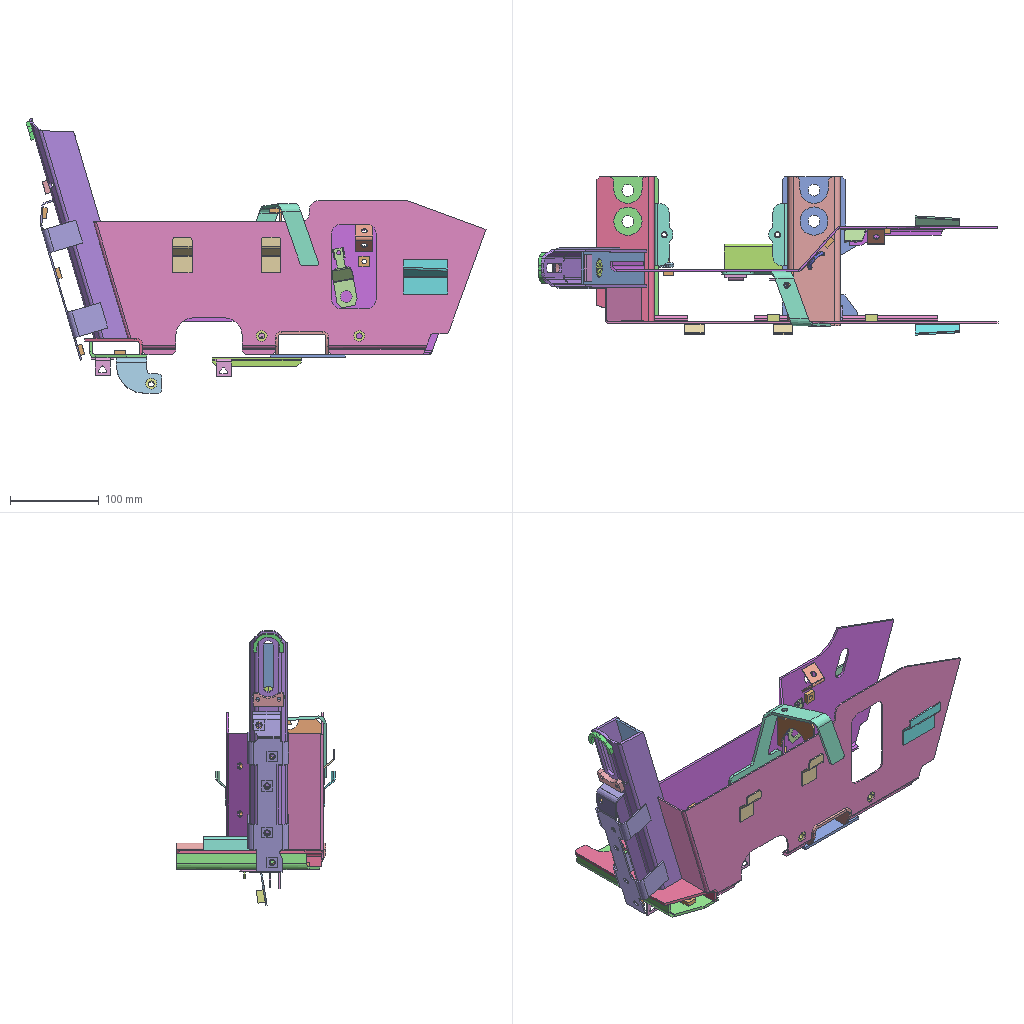Assembly | SolidWorks | 39 different items | 59 placed | box 519 x 179 x 310 mm
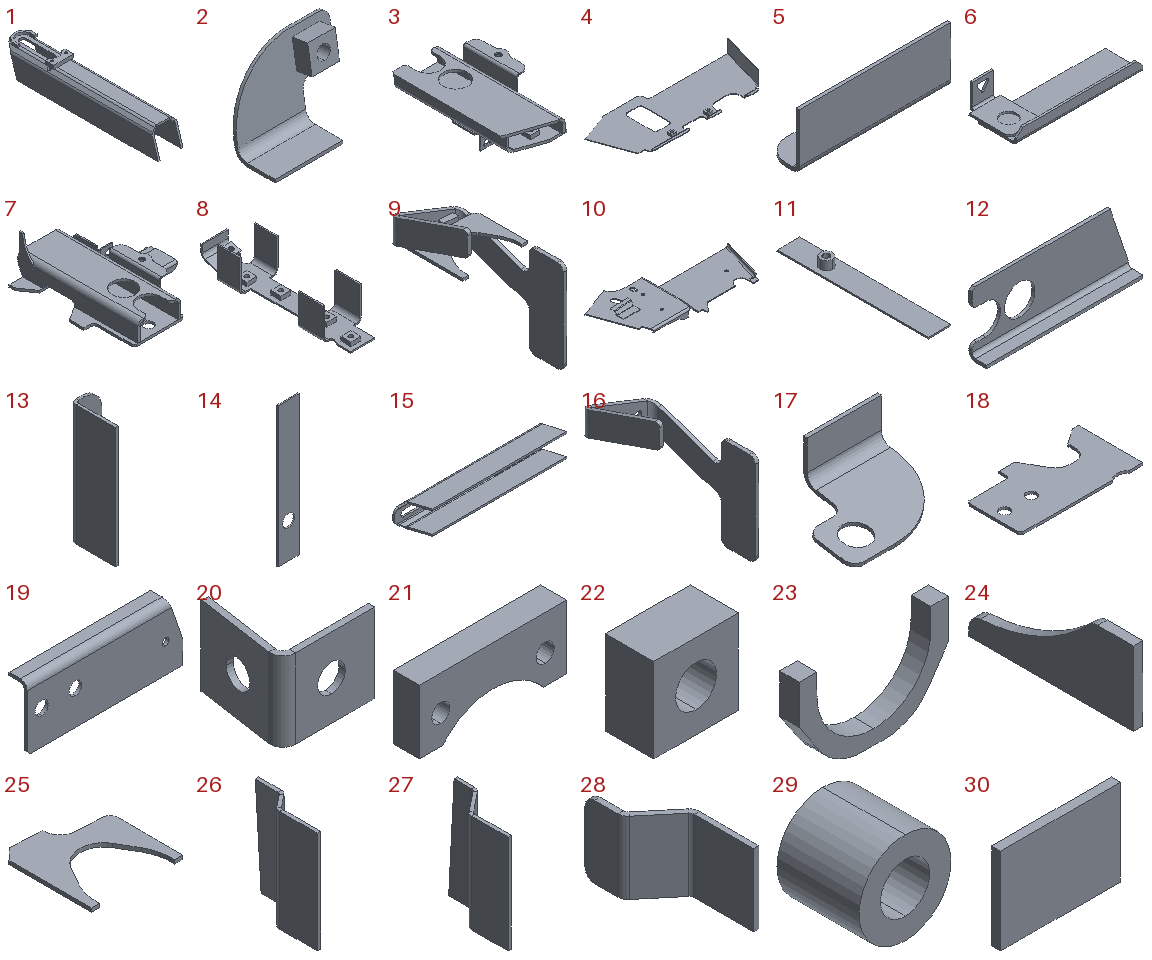Parts list (item | name | quantity | parent item | size | volume | features):
1 | (subassembly) | x1 | - | 42.8 x 270.5 x 50 mm | 92174 mm3 | -
2 | (subassembly) | x1 | in 3 | 51.5 x 26 x 40.249 mm | 4472 mm3 | -
3 | (subassembly) | x1 | - | 87 x 163.6 x 77.249 mm | 83238 mm3 | -
4 | (subassembly) | x1 | - | 442.8 x 174 x 54.1 mm | 103104 mm3 | -
5 | (subassembly) | x2 | in 3, 7 | 70 x 21 x 26 mm | 5040 mm3 | -
6 | (subassembly) | x1 | in 7 | 100 x 40.8 x 21.6 mm | 7480 mm3 | -
7 | (subassembly) | x1 | - | 150 x 168.2 x 79.4 mm | 98058 mm3 | -
8 | (subassembly) | x1 | - | 46 x 182.2 x 40 mm | 19158 mm3 | -
9 | (subassembly) | x1 | - | 61.639 x 95.405 x 122.483 mm | 24396 mm3 | -
10 | (subassembly) | x1 | - | 437.3 x 174 x 67.601 mm | 137259 mm3 | features CompositeCurve 2
11 | (subassembly) | x1 | - | 36.4 x 243 x 18 mm | 24516 mm3 | -
12 | - | x1 | in 3 | 163.6 x 18.8 x 65 mm | 33886 mm3 | features ICE 3, Fillet 2, BreakCorner 1, EdgeFlange 1, FlatPattern 1, SMBaseFlange 1, SheetMetal 1
13 | - | x2 | in 5 | 21 x 26 x 70 mm | 4418 mm3 | features EdgeFlange 1, FlatPattern 1, SMBaseFlange 1, SheetMetal 1
14 | - | x1 | in 11 | 36.4 x 2.3 x 243 mm | 19547 mm3 | features FlatPattern 1, SMBaseFlange 1, SheetMetal 1
15 | - | x1 | in 1 | 270.5 x 44 x 42.8 mm | 88895 mm3 | features Fillet 2, ICE 2, FlatPattern 1, SMBaseFlange 1, SheetMetal 1, UnFold 1
16 | - | x1 | in 9 | 61.639 x 95.405 x 122.483 mm | 19991 mm3 | features EdgeFlange 2, Fillet 2, ICE 2, FlatPattern 1, RefAxis 1, SMBaseFlange 1, SheetMetal 1
17 | - | x1 | in 2 | 51.5 x 40.249 x 26 mm | 3195 mm3 | features Fillet 2, ICE 2, FlatPattern 1, SMBaseFlange 1, SheetMetal 1
18 | - | x1 | in 7 | 161.2 x 85 x 3.2 mm | 34344 mm3 | features Fillet 3, Chamfer 1, FlatPattern 1, SMBaseFlange 1, SheetMetal 1
19 | - | x1 | in 3 | 161.2 x 18.8 x 65 mm | 37684 mm3 | features ICE 3, BreakCorner 1, EdgeFlange 1, FlatPattern 1, SMBaseFlange 1, SheetMetal 1
20 | - | x1 | in 10 | 23.305 x 23.556 x 20 mm | 1295 mm3 | features ICE 2, FlatPattern 1, SMBaseFlange 1, SheetMetal 1
21 | - | x1 | in 1 | 34 x 6 x 14.7 mm | 2300 mm3 | features 3DProfileFeature 1, FlatPattern 1, HoleWzd 1, SMBaseFlange 1, SheetMetal 1
22 | - | x3 | in 2, 4 | 14 x 8 x 14 mm | 1277 mm3 | features FlatPattern 1, HoleWzd 1, SMBaseFlange 1, SheetMetal 1
23 | - | x1 | in 1 | 34 x 4.5 x 21 mm | 979.762 mm3 | features FlatPattern 1, SMBaseFlange 1, SheetMetal 1
24 | - | x1 | in 7 | 2.3 x 40 x 18 mm | 1026 mm3 | features Fillet 1, FlatPattern 1, SMBaseFlange 1, SheetMetal 1
25 | - | x1 | in 9 | 56.8 x 57.632 x 2.3 mm | 3783 mm3 | features BreakCorner 2, FlatPattern 1, SMBaseFlange 1, SheetMetal 1
26 | - | x1 | in 10 | 12.3 x 38.3 x 50.091 mm | 3396 mm3 | features Fillet 2, Blend 1, FlatPattern 1, SheetMetal 1, SolidToSheetMetal 1
27 | - | x1 | in 4 | 13.5 x 39.3 x 50.088 mm | 3525 mm3 | features Fillet 2, Blend 1, FlatPattern 1, SheetMetal 1, SolidToSheetMetal 1
28 | - | x2 | in 4 | 13.1 x 40 x 22 mm | 1581 mm3 | features BreakCorner 1, FlatPattern 1, SMBaseFlange 1, SheetMetal 1
29 | - | x1 | in 11 | 19 x 17 x 19 mm | 3431 mm3 | features Extrusion 1, HoleWzd 1
30 | - | x1 | in 11 | 30.4 x 2.3 x 22 mm | 1538 mm3 | features FlatPattern 1, SMBaseFlange 1, SheetMetal 1
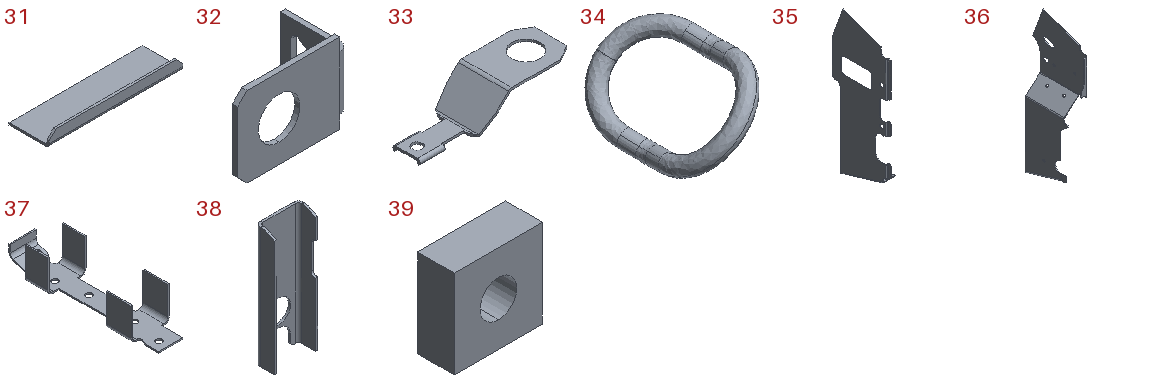31 | - | x1 | in 6 | 100 x 30 x 10 mm | 5946 mm3 | features Chamfer 1, FlatPattern 1, SMBaseFlange 1, SheetMetal 1, UnFold 1
32 | - | x3 | in 3, 6, 7 | 35 x 20 x 25 mm | 1534 mm3 | features ICE 3, Chamfer 1, FlatPattern 1, SMBaseFlange 1, SheetMetal 1
33 | - | x1 | in 10 | 66.449 x 23 x 15.525 mm | 1224 mm3 | features ICE 6, EdgeFlange 2, Hem 2, FlatPattern 1, SMBaseFlange 1, SheetMetal 1
34 | - | x1 | in 10 | 20.665 x 35 x 19.212 mm | 1105 mm3 | features BaseBody 1
35 | - | x1 | in 4 | 40.6 x 174 x 442.8 mm | 93862 mm3 | features Fillet 4, EdgeFlange 3, ICE 2, Chamfer 1, FlatPattern 1, SMBaseFlange 1, SheetMetal 1
36 | - | x1 | in 10 | 50.301 x 174 x 437.3 mm | 127132 mm3 | features EdgeFlange 4, Fillet 4, ICE 2, FlatPattern 1, RefAxis 1, SMBaseFlange 1, SheetMetal 1
37 | - | x1 | in 8 | 46 x 182.2 x 40 mm | 16049 mm3 | features ICE 2, EdgeFlange 1, FlatPattern 1, SMBaseFlange 1, SheetMetal 1
38 | - | x1 | in 7 | 60 x 26.8 x 168.2 mm | 48634 mm3 | features ICE 3, Fillet 2, FlatPattern 1, SMBaseFlange 1, SheetMetal 1, UnFold 1
39 | - | x14 | in 3, 5, 8, 9, 10 | 12 x 5 x 12 mm | 621.825 mm3 | features FlatPattern 1, HoleWzd 1, SMBaseFlange 1, SheetMetal 1
Mates (type | each side: item.copy, entity, surface, feature):
In the top assembly
Coincident | 18.1 face plane Base-Flange1 | 19.1 face plane Base-Flange1
DistanceDim | 38.1 face cylinder Cut-Extrude1 | 12.1 face cylinder Cut-Extrude2
DistanceDim | 12.1 face plane Edge-Flange1 | 38.1 face plane Base-Flange1
Coincident | 18.1 face plane Base-Flange1 | 36.1 face plane Edge-Flange5
Coincident | 38.1 face plane Base-Flange1 | 36.1 face plane Edge-Flange7
DistanceDim | 38.1 face plane Base-Flange1 | 36.1 face plane Base-Flange1
Coincident | 18.1 face plane Base-Flange1 | 35.1 face plane Edge-Flange4
Coincident | 38.1 face plane Base-Flange1 | 35.1 face plane Base-Flange1
DistanceDim | 36.1 face plane Edge-Flange7 | 35.1 face plane Base-Flange1
Coincident | 35.1 face plane Edge-Flange1 | 15.1 face plane Base-Flange1
Coincident | 15.1 face plane Base-Flange1 | 14.1 face plane Base-Flange1
Coincident | 36.1 face plane Edge-Flange8 | 14.1 face plane Base-Flange1
Coincident | 12.1 face plane Base-Flange1 | 14.1 edge
DistanceDim | 14.1 face plane Base-Flange1 | 15.1 face plane Base-Flange1
Coincident | 12.1 face plane Base-Flange1 | 15.1 edge
Coincident | 36.1 face plane Edge-Flange7 | 16.1 face plane Edge-Flange2
Coincident | 15.1 face plane Base-Flange1 | 37.1 face plane Edge-Flange1
Coincident | 15.1 face plane Base-Flange1 | 37.1 face plane Base-Flange1
DistanceDim | 37.1 face plane Base-Flange1 | 21.1 face plane Base-Flange1
DistanceDim | 28.1 face plane Base-Flange2 | 16.1 face cylinder Cut-Extrude2
DistanceDim | 25.1 edge | 36.1 face plane Edge-Flange7
In subassembly 3
Coincident | 19.2 face plane Base-Flange1 | 12.2 face plane Edge-Flange1
Coincident | 19.2 face plane Base-Flange1 | 12.2 face plane Base-Flange1
DistanceDim | 12.2 face plane Edge-Flange1 | 19.2 face plane Base-Flange1
Coincident | 19.2 face plane Base-Flange1 | 39.1 face plane Base-Flange1
Concentric | 19.2 face cylinder Cut-Extrude4 | 39.1 face cylinder M6 Tapped Hole1
Parallel | 19.2 face plane Base-Flange1 | 39.1 face plane Base-Flange1
Coincident | 19.2 face plane Base-Flange1 | 32.1 face plane Base-Flange1
DistanceDim | 32.1 face cylinder Cut-Extrude3 | 19.2 face plane Edge-Flange1
DistanceDim | 32.1 face cylinder Cut-Extrude3 | 19.2 face plane Base-Flange1
Parallel | 19.2 face plane Base-Flange1 | 32.1 face plane Base-Flange1
Coincident | 19.2 face plane Base-Flange1 | 17.1 face plane Base-Flange1
DistanceDim | 17.1 face plane Base-Flange1 | 19.2 face plane Base-Flange1
DistanceDim | 17.1 face plane Base-Flange1 | 19.2 face plane Edge-Flange1
Coincident | 12.2 face plane Edge-Flange1 | 13.1 face plane Edge-Flange1
DistanceDim | 13.1 edge | 19.2 face plane Base-Flange1
DistanceDim | 12.2 face plane Edge-Flange1 | 13.1 face cylinder Base-Flange1
In subassembly 2
Coincident | 17.2 face plane Base-Flange1 | 22.1 face plane Base-Flange1
Concentric | 17.2 face cylinder Cut-Extrude2 | 22.1 face cylinder M8 Tapped Hole1
Parallel | 17.2 face plane Base-Flange1 | 22.1 face plane Base-Flange1
In subassembly 5
Coincident | 13.2 face plane Base-Flange1 | 39.1 face plane Base-Flange1
Concentric | 13.2 face cylinder Base-Flange1 | 39.1 face cylinder M6 Tapped Hole1
Parallel | 13.2 face plane Edge-Flange1 | 39.1 face plane Base-Flange1
In subassembly 7
Coincident | 38.2 face plane Base-Flange1 | 18.2 face plane Base-Flange1 | 2 times
DistanceDim | 38.2 face plane Base-Flange1 | 18.2 face plane Base-Flange1
Coincident | 18.2 face plane Base-Flange1 | 31.1 face plane Base-Flange1
DistanceDim | 31.1 face plane Base-Flange1 | 18.2 face plane Base-Flange1
DistanceDim | 18.2 face plane Base-Flange1 | 31.1 face plane Base-Flange1
Coincident | 38.2 face plane Base-Flange1 | 32.1 face plane Base-Flange1
DistanceDim | 38.2 face plane Base-Flange1 | 32.1 face cylinder Cut-Extrude3
DistanceDim | 18.2 face plane Base-Flange1 | 32.1 face plane Base-Flange1
Coincident | 38.2 face plane Base-Flange1 | 13.1 face plane Edge-Flange1
DistanceDim | 38.2 face plane Base-Flange1 | 13.1 face cylinder Base-Flange1
DistanceDim | 13.1 edge | 18.2 face plane Base-Flange1
Coincident | 38.2 face plane Base-Flange1 | 24.1 face plane Base-Flange1
DistanceDim | 18.2 face plane Base-Flange1 | 24.1 face plane Base-Flange1
DistanceDim | 24.1 face plane Base-Flange1 | 38.2 face plane Base-Flange1
In subassembly 6
Coincident | 31.2 face plane Base-Flange1 | 32.1 face plane Base-Flange1 | 2 times
DistanceDim | 32.1 face cylinder Cut-Extrude3 | 31.2 face plane Base-Flange1
In subassembly 10
Coincident | 36.2 face plane Base-Flange1 | 39.1 face plane Base-Flange1
Concentric | 36.2 face cylinder Base-Flange1 | 39.1 face cylinder M6 Tapped Hole1
Parallel | 36.2 face plane Edge-Flange5 | 39.1 face plane Base-Flange1
Coincident | 36.2 face plane Base-Flange1 | 39.2 face plane Base-Flange1
Concentric | 36.2 face cylinder Base-Flange1 | 39.2 face cylinder M6 Tapped Hole1
Parallel | 39.1 face plane Base-Flange1 | 39.2 face plane Base-Flange1
Coincident | 36.2 face plane Edge-Flange7 | 39.3 face plane Base-Flange1
Concentric | 36.2 face cylinder Cut-Extrude2 | 39.3 face cylinder M6 Tapped Hole1
Parallel | 36.2 face plane Edge-Flange5 | 39.3 face plane Base-Flange1
Coincident | 36.2 face plane Edge-Flange6 | 39.4 face plane Base-Flange1
Concentric | 36.2 face cylinder Cut-Extrude1 | 39.4 face cylinder M6 Tapped Hole1
Coincident | 36.2 face plane Edge-Flange6 | 39.5 face plane Base-Flange1
Concentric | 36.2 face cylinder Cut-Extrude1 | 39.5 face cylinder M6 Tapped Hole1
Parallel | 39.4 face plane Base-Flange1 | 39.5 face plane Base-Flange1
Parallel | 39.4 face plane Base-Flange1 | 36.2 face plane Edge-Flange6
Coincident | 36.2 face plane Base-Flange1 | 26.1 face plane Convert-Entities1
DistanceDim | 36.2 face plane Edge-Flange5 | 26.1 face plane Convert-Entities1
DistanceDim | 36.2 face plane Base-Flange1 | 26.1 face plane Convert-Entities1
Coincident | 36.2 face plane Base-Flange1 | 20.1 edge | 2 times
DistanceDim | 36.2 face plane Base-Flange1 | 20.1 edge
DistanceDim | 20.1 face plane Base-Flange1 | 39.1 face cylinder M6 Tapped Hole1
Coincident | 36.2 face plane Edge-Flange6 | 34.1 edge
Tangent | 36.2 face plane Edge-Flange6 | 34.1 face surface:4006 Base Body
DistanceDim | 39.4 face cylinder M6 Tapped Hole1 | 10.1 plane
Parallel | 39.4 face plane Base-Flange1 | 10.1 plane
DistanceDim | 39.4 face plane Base-Flange1 | 34.1 edge
Coincident | 36.2 face plane Base-Flange1 | 33.1 face plane Base-Flange1
DistanceDim | 20.1 face plane Base-Flange1 | 33.1 face cylinder Base-Flange1
DistanceDim | 33.1 face cylinder Base-Flange1 | 36.2 face plane Base-Flange1
PlanarAngleDim | 20.1 face plane Base-Flange1 | 33.1 face plane Base-Flange1
In subassembly 4
Coincident | 35.2 face plane Base-Flange1 | 27.1 face plane Convert-Entities1
DistanceDim | 27.1 face plane Convert-Entities1 | 35.2 face plane Edge-Flange4
DistanceDim | 35.2 face plane Edge-Flange3 | 27.1 face plane Convert-Entities1
Coincident | 35.2 face plane Base-Flange1 | 28.2 face plane Base-Flange2
DistanceDim | 27.1 face plane Convert-Entities1 | 28.2 face plane Base-Flange2 | 2 times
Coincident | 35.2 face plane Base-Flange1 | 28.3 face plane Base-Flange2
DistanceDim | 28.2 face plane Base-Flange2 | 28.3 face plane Base-Flange2
Coincident | 28.2 face plane Base-Flange2 | 28.3 face plane Base-Flange2
Coincident | 35.2 face plane Base-Flange1 | 22.1 face plane Base-Flange1
Concentric | 35.2 face cylinder Cut-Extrude2 | 22.1 face cylinder M8 Tapped Hole1
Parallel | 35.2 face plane Edge-Flange4 | 22.1 face plane Base-Flange1
Concentric | 35.2 face cylinder Cut-Extrude2 | 22.2 face cylinder M8 Tapped Hole1
Coincident | 35.2 face plane Base-Flange1 | 22.2 face plane Base-Flange1
Coincident | 22.1 face plane Base-Flange1 | 22.2 face plane Base-Flange1
In subassembly 1
Coincident | 15.2 plane | 23.1 plane
Coincident | 15.2 face plane Base-Flange1 | 23.1 face plane Base-Flange1
DistanceDim | 15.2 face plane Base-Flange1 | 23.1 face plane Base-Flange1
Coincident | 15.2 face plane Base-Flange1 | 21.2 face plane Base-Flange1
Coincident | 15.2 plane | 21.2 plane
DistanceDim | 15.2 edge | 21.2 edge
In subassembly 11
Concentric | 14.2 face cylinder Base-Flange1 | 29.1 face cylinder Boss-Extrude1
DistanceDim | 29.1 face plane Boss-Extrude1 | 14.2 face plane Base-Flange1
Coincident | 14.2 face plane Base-Flange1 | 30.1 face plane Base-Flange1
Coincident | 14.2 plane | 30.1 plane
DistanceDim | 30.1 face plane Base-Flange1 | 14.2 face plane Base-Flange1
In subassembly 9
DistanceDim | 16.2 face cylinder Cut-Extrude2 | 25.2 face plane Base-Flange1
Parallel | 16.2 face plane Edge-Flange2 | 25.2 face plane Base-Flange1
Coincident | 16.2 face plane Edge-Flange2 | 25.2 face plane Base-Flange1
Coincident | 16.2 face plane Base-Flange2 | 25.2 edge
Coincident | 16.2 face plane Base-Flange2 | 39.1 face plane Base-Flange1
Concentric | 16.2 face cylinder Cut-Extrude2 | 39.1 face cylinder M6 Tapped Hole1
Parallel | 16.2 face plane Edge-Flange2 | 39.1 face plane Base-Flange1
In subassembly 8
Coincident | 37.2 face plane Base-Flange1 | 39.1 face plane Base-Flange1
Concentric | 37.2 face cylinder Cut-Extrude1 | 39.1 face cylinder M6 Tapped Hole1
Coincident | 37.2 face plane Base-Flange1 | 39.2 face plane Base-Flange1
Concentric | 37.2 face cylinder Cut-Extrude1 | 39.2 face cylinder M6 Tapped Hole1
Coincident | 37.2 face plane Base-Flange1 | 39.3 face plane Base-Flange1
Concentric | 37.2 face cylinder Cut-Extrude1 | 39.3 face cylinder M6 Tapped Hole1
Coincident | 37.2 face plane Base-Flange1 | 39.4 face plane Base-Flange1
Concentric | 37.2 face cylinder Cut-Extrude1 | 39.4 face cylinder M6 Tapped Hole1
Coincident | 37.2 face plane Base-Flange1 | 39.5 face plane Base-Flange1
Concentric | 37.2 face cylinder Cut-Extrude2 | 39.5 face cylinder M6 Tapped Hole1
Parallel | 37.2 face plane Cut-Extrude1 | 39.5 face plane Base-Flange1
Parallel | 39.1 face plane Base-Flange1 | 39.5 face plane Base-Flange1
Parallel | 37.2 face plane Edge-Flange1 | 39.2 face plane Base-Flange1
Parallel | 37.2 face plane Edge-Flange1 | 39.3 face plane Base-Flange1
Parallel | 37.2 face plane Cut-Extrude1 | 39.4 face plane Base-Flange1